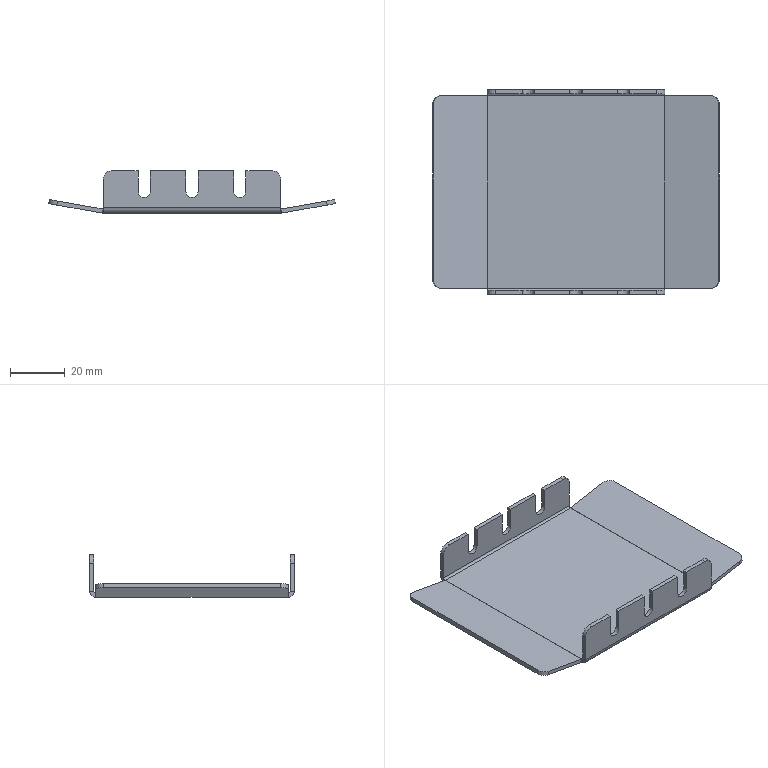Part | STEP file | 1 solid | 70 faces | box 104.913 x 75 x 15.5 mm | volume 13779 mm3 | plane 48 | cylinder 22 | commonest cylinder face diameters 6 x8 4.5 x6 1.473 x4 4.473 x4